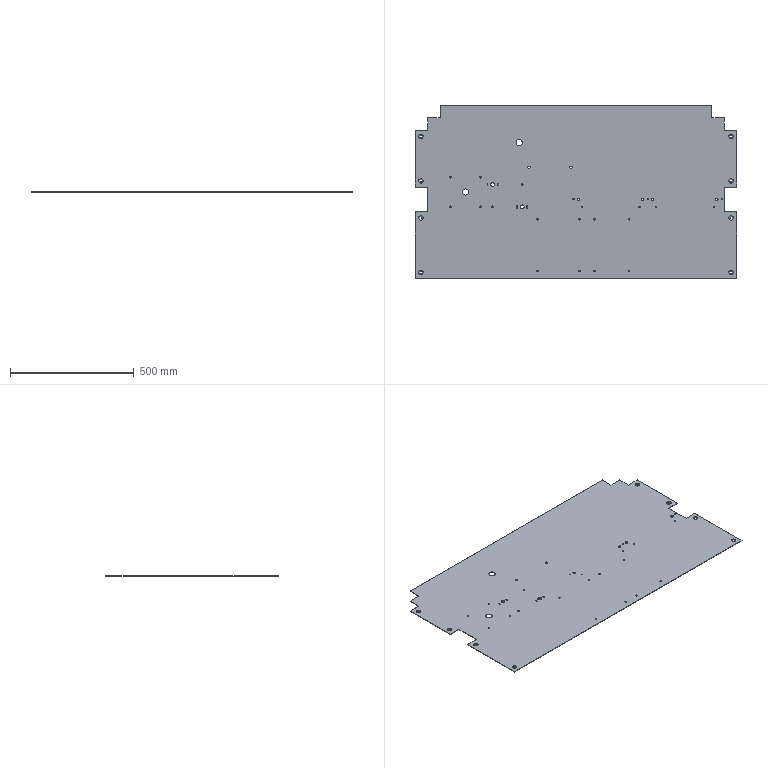Part | STEP file | 1300 table top 2 | 1 solid | 116 faces | box 1300 x 700 x 2 mm | volume 1762203 mm3 | cylinder 78 | plane 22 | cone 16 | commonest cylinder face diameters 6.8 x28 3.3 x16 5 x14 10 x12 15 x4 25.5 x4